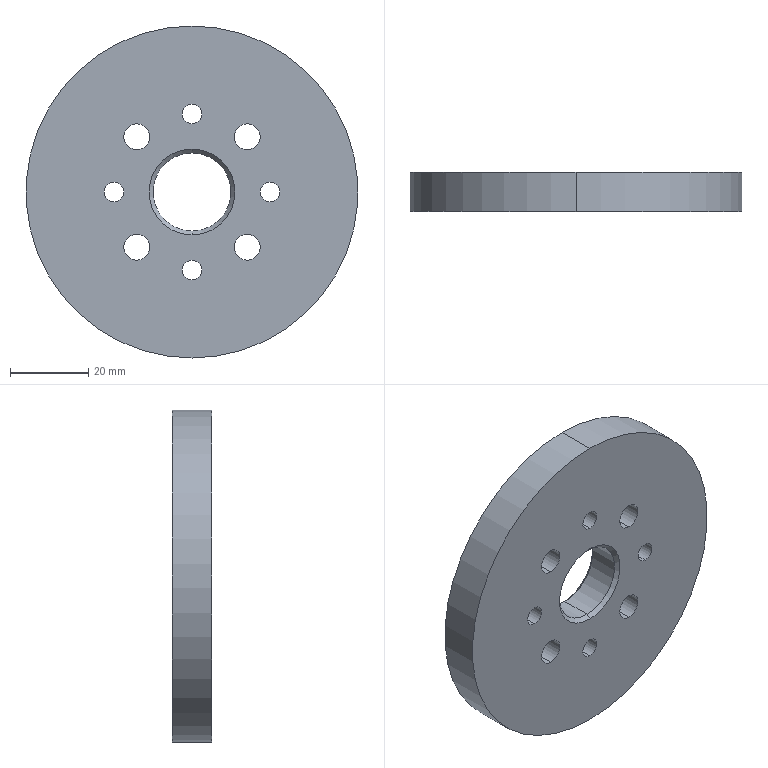Part | STEP file | 0229_214_Holder | 1 solid | 26 faces | box 85 x 10 x 85 mm | volume 51385 mm3 | cylinder 20 | cone 4 | plane 2 | commonest cylinder face diameters 5 x8 6.6 x8 20 x2 85 x2